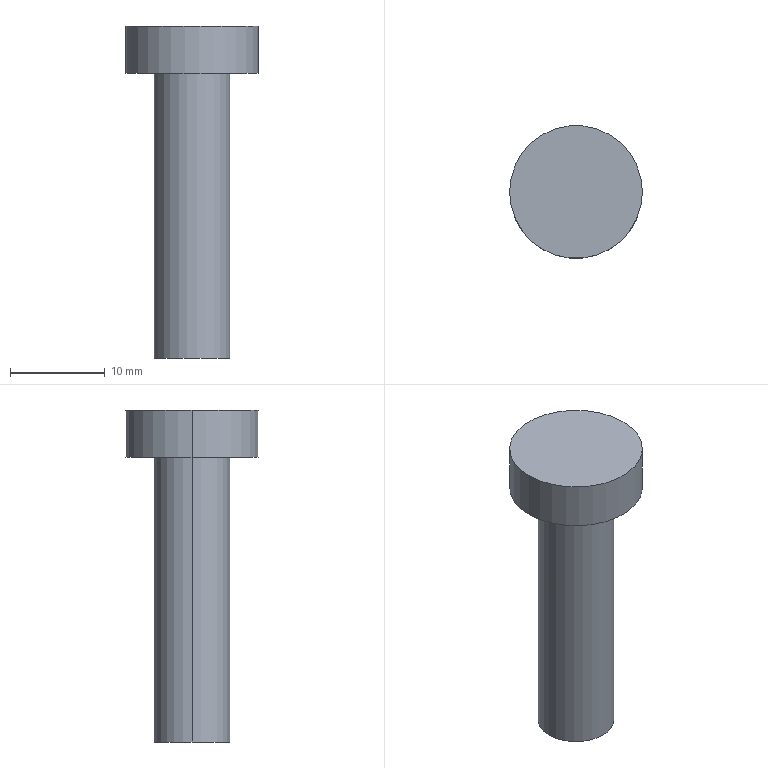Part | Creo | 1 solid | 7 faces | box 14 x 14 x 35 mm | volume 2278 mm3 | cylinder 4 | plane 3 | commonest cylinder face diameters 8 x2 14 x2
STEP:
#1=CARTESIAN_POINT('',(64.147,173.569,-270.5));
#2=VERTEX_POINT('',#1);
#3=CARTESIAN_POINT('',(56.147,173.569,-270.5));
#4=VERTEX_POINT('',#3);
#5=CARTESIAN_POINT('',(60.147,173.569,-270.5));
#6=DIRECTION('',(0.,0.,-1.));
#7=DIRECTION('',(1.,0.,0.));
#8=AXIS2_PLACEMENT_3D('',#5,#6,#7);
#9=CIRCLE('',#8,4.);
#10=EDGE_CURVE('',#2,#4,#9,.T.);
#11=ORIENTED_EDGE('',*,*,#10,.T.);
#12=CARTESIAN_POINT('',(56.147,173.569,-240.5));
#13=VERTEX_POINT('',#12);
#14=CARTESIAN_POINT('',(56.147,173.569,-270.5));
#15=DIRECTION('',(0.,0.,1.));
#16=VECTOR('',#15,30.);
#17=LINE('',#14,#16);
#18=EDGE_CURVE('',#4,#13,#17,.T.);
#19=ORIENTED_EDGE('',*,*,#18,.T.);
#20=CARTESIAN_POINT('',(64.147,173.569,-240.5));
#21=VERTEX_POINT('',#20);
#22=CARTESIAN_POINT('',(60.147,173.569,-240.5));
#23=DIRECTION('',(0.,0.,1.));
#24=DIRECTION('',(-1.,0.,0.));
#25=AXIS2_PLACEMENT_3D('',#22,#23,#24);
#26=CIRCLE('',#25,4.);
#27=EDGE_CURVE('',#13,#21,#26,.T.);
#28=ORIENTED_EDGE('',*,*,#27,.T.);
#29=CARTESIAN_POINT('',(64.147,173.569,-270.5));
#30=DIRECTION('',(0.,0.,1.));
#31=VECTOR('',#30,30.);
#32=LINE('',#29,#31);
#33=EDGE_CURVE('',#2,#21,#32,.T.);
#34=ORIENTED_EDGE('',*,*,#33,.F.);
#35=EDGE_LOOP('',(#11,#19,#28,#34));
#36=FACE_OUTER_BOUND('',#35,.F.);
#37=CARTESIAN_POINT('',(60.147,173.569,-520.5));
#38=DIRECTION('',(0.,0.,1.));
#39=DIRECTION('',(-1.,0.,0.));
#40=AXIS2_PLACEMENT_3D('',#37,#38,#39);
#41=CYLINDRICAL_SURFACE('',#40,4.);
#42=ADVANCED_FACE('',(#36),#41,.T.);
#43=CARTESIAN_POINT('',(60.147,173.569,-270.5));
#44=DIRECTION('',(0.,0.,-1.));
#45=DIRECTION('',(-1.,0.,0.));
#46=AXIS2_PLACEMENT_3D('',#43,#44,#45);
#47=CIRCLE('',#46,4.);
#48=EDGE_CURVE('',#4,#2,#47,.T.);
#49=ORIENTED_EDGE('',*,*,#48,.F.);
#50=ORIENTED_EDGE('',*,*,#10,.F.);
#51=EDGE_LOOP('',(#49,#50));
#52=FACE_OUTER_BOUND('',#51,.F.);
#53=CARTESIAN_POINT('',(-231.81,-52.862,-270.5));
#54=DIRECTION('',(0.,0.,-1.));
#55=DIRECTION('',(-1.,0.,0.));
#56=AXIS2_PLACEMENT_3D('',#53,#54,#55);
#57=PLANE('',#56);
#58=ADVANCED_FACE('',(#52),#57,.T.);
#59=ORIENTED_EDGE('',*,*,#48,.T.);
#60=ORIENTED_EDGE('',*,*,#33,.T.);
#61=CARTESIAN_POINT('',(60.147,173.569,-240.5));
#62=DIRECTION('',(0.,0.,1.));
#63=DIRECTION('',(1.,0.,0.));
#64=AXIS2_PLACEMENT_3D('',#61,#62,#63);
#65=CIRCLE('',#64,4.);
#66=EDGE_CURVE('',#21,#13,#65,.T.);
#67=ORIENTED_EDGE('',*,*,#66,.T.);
#68=ORIENTED_EDGE('',*,*,#18,.F.);
#69=EDGE_LOOP('',(#59,#60,#67,#68));
#70=FACE_OUTER_BOUND('',#69,.F.);
#71=CARTESIAN_POINT('',(60.147,173.569,-520.5));
#72=DIRECTION('',(0.,0.,1.));
#73=DIRECTION('',(-1.,0.,0.));
#74=AXIS2_PLACEMENT_3D('',#71,#72,#73);
#75=CYLINDRICAL_SURFACE('',#74,4.);
#76=ADVANCED_FACE('',(#70),#75,.T.);
#77=CARTESIAN_POINT('',(53.147,173.569,-240.5));
#78=VERTEX_POINT('',#77);
#79=CARTESIAN_POINT('',(67.147,173.569,-240.5));
#80=VERTEX_POINT('',#79);
#81=CARTESIAN_POINT('',(60.147,173.569,-240.5));
#82=DIRECTION('',(0.,0.,-1.));
#83=DIRECTION('',(-1.,0.,0.));
#84=AXIS2_PLACEMENT_3D('',#81,#82,#83);
#85=CIRCLE('',#84,7.);
#86=EDGE_CURVE('',#78,#80,#85,.T.);
#87=ORIENTED_EDGE('',*,*,#86,.F.);
#88=CARTESIAN_POINT('',(60.147,173.569,-240.5));
#89=DIRECTION('',(0.,0.,-1.));
#90=DIRECTION('',(1.,0.,0.));
#91=AXIS2_PLACEMENT_3D('',#88,#89,#90);
#92=CIRCLE('',#91,7.);
#93=EDGE_CURVE('',#80,#78,#92,.T.);
#94=ORIENTED_EDGE('',*,*,#93,.F.);
#95=EDGE_LOOP('',(#87,#94));
#96=FACE_OUTER_BOUND('',#95,.F.);
#97=ORIENTED_EDGE('',*,*,#27,.F.);
#98=ORIENTED_EDGE('',*,*,#66,.F.);
#99=EDGE_LOOP('',(#97,#98));
#100=FACE_BOUND('',#99,.F.);
#101=CARTESIAN_POINT('',(60.147,173.569,-240.5));
#102=DIRECTION('',(0.,0.,1.));
#103=DIRECTION('',(-1.,0.,0.));
#104=AXIS2_PLACEMENT_3D('',#101,#102,#103);
#105=PLANE('',#104);
#106=ADVANCED_FACE('',(#96,#100),#105,.F.);
#107=CARTESIAN_POINT('',(67.147,173.569,-235.5));
#108=VERTEX_POINT('',#107);
#109=CARTESIAN_POINT('',(53.147,173.569,-235.5));
#110=VERTEX_POINT('',#109);
#111=CARTESIAN_POINT('',(60.147,173.569,-235.5));
#112=DIRECTION('',(0.,0.,1.));
#113=DIRECTION('',(1.,0.,0.));
#114=AXIS2_PLACEMENT_3D('',#111,#112,#113);
#115=CIRCLE('',#114,7.);
#116=EDGE_CURVE('',#108,#110,#115,.T.);
#117=ORIENTED_EDGE('',*,*,#116,.T.);
#118=CARTESIAN_POINT('',(53.147,173.569,-240.5));
#119=DIRECTION('',(0.,0.,1.));
#120=VECTOR('',#119,5.);
#121=LINE('',#118,#120);
#122=EDGE_CURVE('',#78,#110,#121,.T.);
#123=ORIENTED_EDGE('',*,*,#122,.F.);
#124=ORIENTED_EDGE('',*,*,#86,.T.);
#125=CARTESIAN_POINT('',(67.147,173.569,-240.5));
#126=DIRECTION('',(0.,0.,1.));
#127=VECTOR('',#126,5.);
#128=LINE('',#125,#127);
#129=EDGE_CURVE('',#80,#108,#128,.T.);
#130=ORIENTED_EDGE('',*,*,#129,.T.);
#131=EDGE_LOOP('',(#117,#123,#124,#130));
#132=FACE_OUTER_BOUND('',#131,.F.);
#133=CARTESIAN_POINT('',(60.147,173.569,-225.087));
#134=DIRECTION('',(0.,0.,1.));
#135=DIRECTION('',(-1.,0.,0.));
#136=AXIS2_PLACEMENT_3D('',#133,#134,#135);
#137=CYLINDRICAL_SURFACE('',#136,7.);
#138=ADVANCED_FACE('',(#132),#137,.T.);
#139=CARTESIAN_POINT('',(60.147,173.569,-235.5));
#140=DIRECTION('',(0.,0.,1.));
#141=DIRECTION('',(-1.,0.,0.));
#142=AXIS2_PLACEMENT_3D('',#139,#140,#141);
#143=CIRCLE('',#142,7.);
#144=EDGE_CURVE('',#110,#108,#143,.T.);
#145=ORIENTED_EDGE('',*,*,#144,.F.);
#146=ORIENTED_EDGE('',*,*,#116,.F.);
#147=EDGE_LOOP('',(#145,#146));
#148=FACE_OUTER_BOUND('',#147,.F.);
#149=CARTESIAN_POINT('',(64.147,173.569,-235.5));
#150=DIRECTION('',(0.,0.,-1.));
#151=DIRECTION('',(1.,0.,0.));
#152=AXIS2_PLACEMENT_3D('',#149,#150,#151);
#153=PLANE('',#152);
#154=ADVANCED_FACE('',(#148),#153,.F.);
#155=ORIENTED_EDGE('',*,*,#144,.T.);
#156=ORIENTED_EDGE('',*,*,#129,.F.);
#157=ORIENTED_EDGE('',*,*,#93,.T.);
#158=ORIENTED_EDGE('',*,*,#122,.T.);
#159=EDGE_LOOP('',(#155,#156,#157,#158));
#160=FACE_OUTER_BOUND('',#159,.F.);
#161=CARTESIAN_POINT('',(60.147,173.569,-225.087));
#162=DIRECTION('',(0.,0.,1.));
#163=DIRECTION('',(-1.,0.,0.));
#164=AXIS2_PLACEMENT_3D('',#161,#162,#163);
#165=CYLINDRICAL_SURFACE('',#164,7.);
#166=ADVANCED_FACE('',(#160),#165,.T.);
#167=CLOSED_SHELL('',(#42,#58,#76,#106,#138,#154,#166));
#168=MANIFOLD_SOLID_BREP('',#167);
#169=(LENGTH_UNIT()NAMED_UNIT(*)SI_UNIT(.MILLI.,.METRE.));
#170=UNCERTAINTY_MEASURE_WITH_UNIT(LENGTH_MEASURE(0.004021),#169,'','');
#171=(NAMED_UNIT(*)PLANE_ANGLE_UNIT()SI_UNIT($,.RADIAN.));
#172=PLANE_ANGLE_MEASURE_WITH_UNIT(PLANE_ANGLE_MEASURE(0.01745),#171);
#173=(CONVERSION_BASED_UNIT('DEGREE',#172)NAMED_UNIT(*)PLANE_ANGLE_UNIT());
#174=(NAMED_UNIT(*)SI_UNIT($,.STERADIAN.)SOLID_ANGLE_UNIT());
#175=(GEOMETRIC_REPRESENTATION_CONTEXT(3)GLOBAL_UNCERTAINTY_ASSIGNED_CONTEXT((#170))GLOBAL_UNIT_ASSIGNED_CONTEXT((#169,#173,#174))REPRESENTATION_CONTEXT('',''));
#176=ADVANCED_BREP_SHAPE_REPRESENTATION('',(#168),#175);